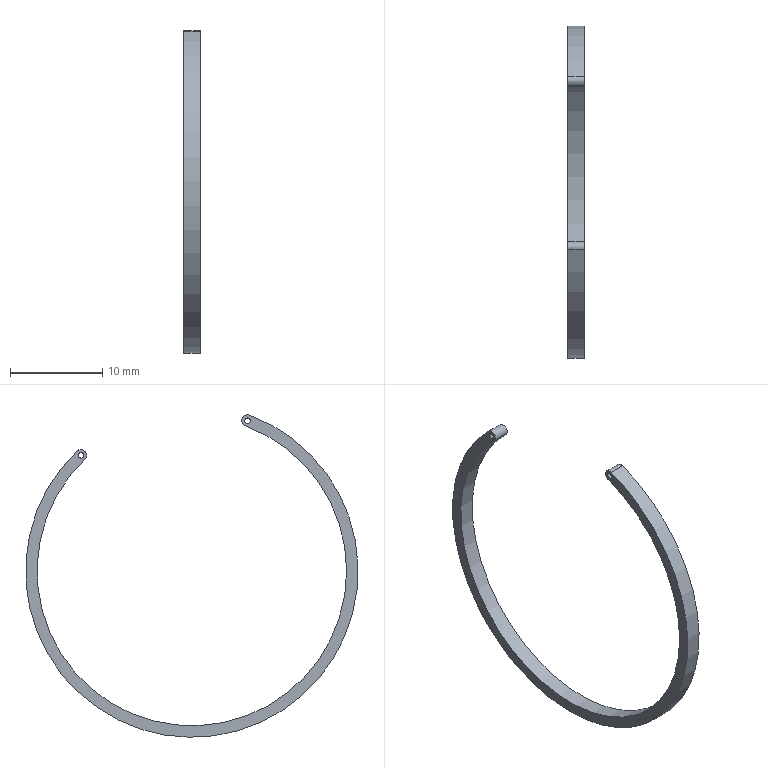Part | STEP file | Snap Ring_Bala35 | 1 solid | 10 faces | box 1.75 x 36 x 34.918 mm | volume 197.431 mm3 | cylinder 6 | spline 2 | plane 2 | commonest cylinder face diameters 0.6 x4 33.5 x1 36 x1